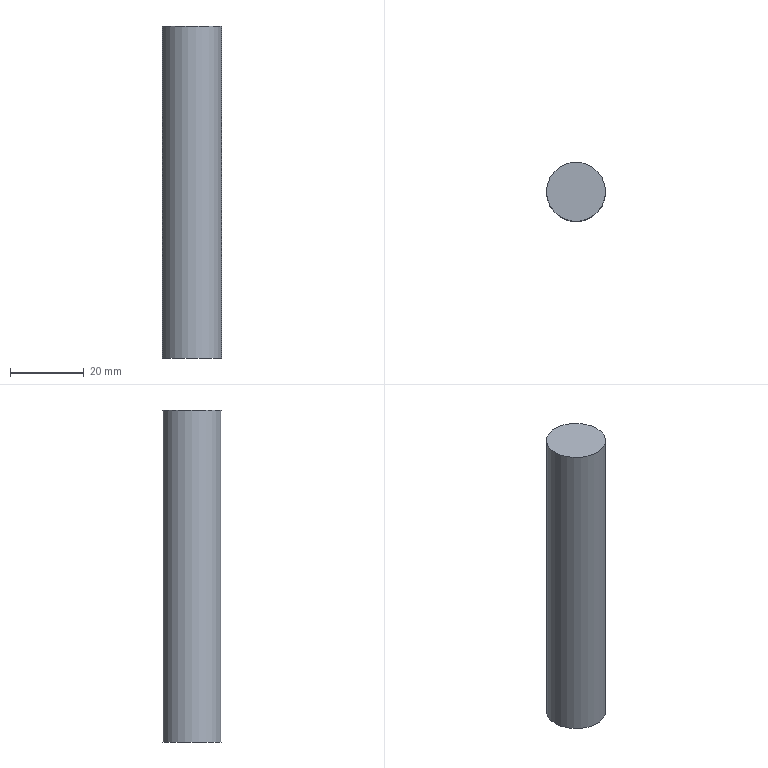Part | STEP file | solid 218 | 1 solid | 3 faces | box 16 x 16 x 90 mm | volume 18096 mm3 | plane 2 | cylinder 1 | commonest cylinder face diameters 16 x1